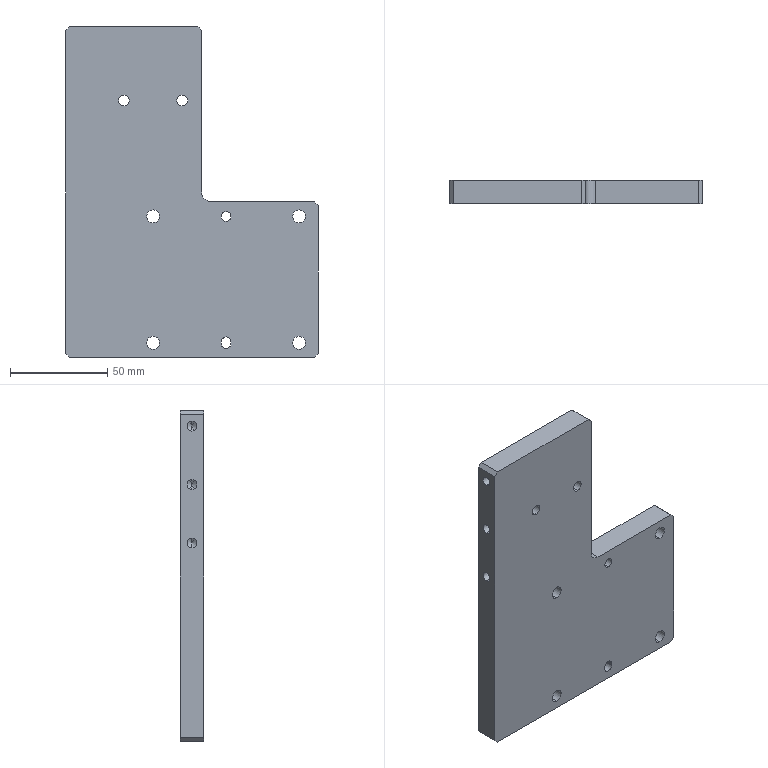Part | SolidWorks | features HoleWzd 5, Chamfer 1, Extrusion 1 | 1 solid | 63 faces | box 130 x 12 x 170 mm | volume 194409 mm3 | cylinder 36 | plane 21 | cone 6 | commonest cylinder face diameters 5 x11 6.6 x8 11 x8 10 x5 5.5 x4